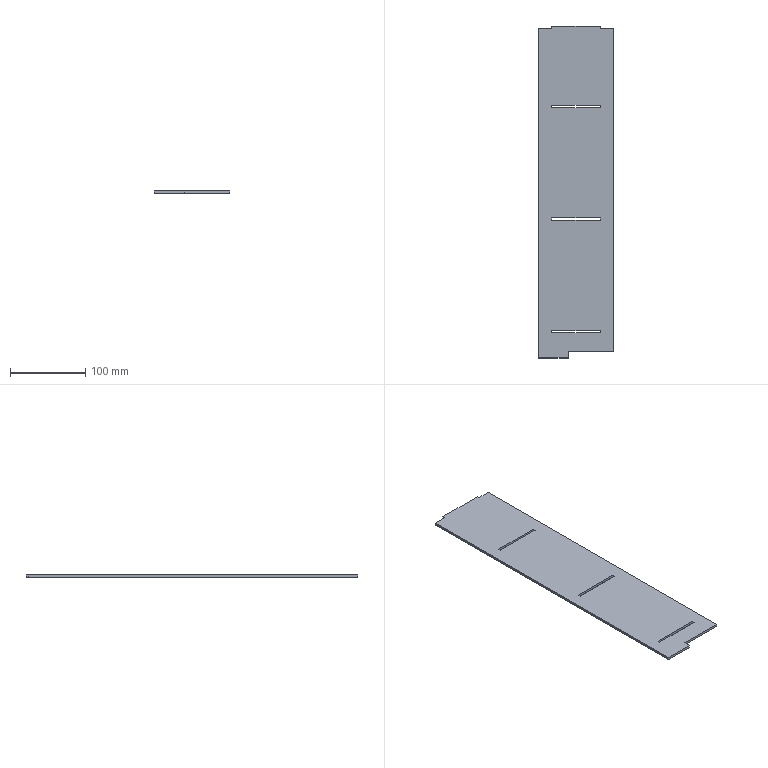Part | SolidWorks | features FlatPattern 1, SMBaseFlange 1, SheetMetal 1 | 1 solid | 24 faces | box 100 x 442 x 3.2 mm | volume 137506 mm3 | plane 24
STEP:
#1=CARTESIAN_POINT('',(72.5,-36.2,3.2));
#2=VERTEX_POINT('',#1);
#3=CARTESIAN_POINT('',(72.5,-33.,3.2));
#4=VERTEX_POINT('',#3);
#5=CARTESIAN_POINT('',(72.5,-33.,3.2));
#6=DIRECTION('',(0.,1.,0.));
#7=VECTOR('',#6,1000.);
#8=LINE('',#5,#7);
#9=EDGE_CURVE('',#2,#4,#8,.T.);
#10=ORIENTED_EDGE('',*,*,#9,.F.);
#11=CARTESIAN_POINT('',(7.5,-36.2,3.2));
#12=VERTEX_POINT('',#11);
#13=CARTESIAN_POINT('',(72.5,-36.2,3.2));
#14=DIRECTION('',(1.,0.,0.));
#15=VECTOR('',#14,1000.);
#16=LINE('',#13,#15);
#17=EDGE_CURVE('',#12,#2,#16,.T.);
#18=ORIENTED_EDGE('',*,*,#17,.F.);
#19=CARTESIAN_POINT('',(7.5,-33.,3.2));
#20=VERTEX_POINT('',#19);
#21=CARTESIAN_POINT('',(7.5,-33.,3.2));
#22=DIRECTION('',(0.,-1.,0.));
#23=VECTOR('',#22,1000.);
#24=LINE('',#21,#23);
#25=EDGE_CURVE('',#20,#12,#24,.T.);
#26=ORIENTED_EDGE('',*,*,#25,.F.);
#27=CARTESIAN_POINT('',(72.5,-33.,3.2));
#28=DIRECTION('',(-1.,0.,0.));
#29=VECTOR('',#28,1000.);
#30=LINE('',#27,#29);
#31=EDGE_CURVE('',#4,#20,#30,.T.);
#32=ORIENTED_EDGE('',*,*,#31,.F.);
#33=EDGE_LOOP('',(#10,#18,#26,#32));
#34=FACE_BOUND('',#33,.T.);
#35=CARTESIAN_POINT('',(7.5,222.5,3.2));
#36=VERTEX_POINT('',#35);
#37=CARTESIAN_POINT('',(7.5,219.5,3.2));
#38=VERTEX_POINT('',#37);
#39=CARTESIAN_POINT('',(7.5,219.5,3.2));
#40=DIRECTION('',(0.,-1.,0.));
#41=VECTOR('',#40,1000.);
#42=LINE('',#39,#41);
#43=EDGE_CURVE('',#36,#38,#42,.T.);
#44=ORIENTED_EDGE('',*,*,#43,.T.);
#45=CARTESIAN_POINT('',(-10.,219.5,3.2));
#46=VERTEX_POINT('',#45);
#47=CARTESIAN_POINT('',(-10.,219.5,3.2));
#48=DIRECTION('',(-1.,0.,0.));
#49=VECTOR('',#48,1000.);
#50=LINE('',#47,#49);
#51=EDGE_CURVE('',#38,#46,#50,.T.);
#52=ORIENTED_EDGE('',*,*,#51,.T.);
#53=CARTESIAN_POINT('',(-10.,-219.5,3.2));
#54=VERTEX_POINT('',#53);
#55=CARTESIAN_POINT('',(-10.,-219.5,3.2));
#56=DIRECTION('',(0.,-1.,0.));
#57=VECTOR('',#56,1000.);
#58=LINE('',#55,#57);
#59=EDGE_CURVE('',#46,#54,#58,.T.);
#60=ORIENTED_EDGE('',*,*,#59,.T.);
#61=CARTESIAN_POINT('',(29.7,-219.5,3.2));
#62=VERTEX_POINT('',#61);
#63=CARTESIAN_POINT('',(29.7,-219.5,3.2));
#64=DIRECTION('',(1.,0.,0.));
#65=VECTOR('',#64,1000.);
#66=LINE('',#63,#65);
#67=EDGE_CURVE('',#54,#62,#66,.T.);
#68=ORIENTED_EDGE('',*,*,#67,.T.);
#69=CARTESIAN_POINT('',(29.7,-211.2,3.2));
#70=VERTEX_POINT('',#69);
#71=CARTESIAN_POINT('',(29.7,-211.2,3.2));
#72=DIRECTION('',(0.,1.,0.));
#73=VECTOR('',#72,1000.);
#74=LINE('',#71,#73);
#75=EDGE_CURVE('',#62,#70,#74,.T.);
#76=ORIENTED_EDGE('',*,*,#75,.T.);
#77=CARTESIAN_POINT('',(90.,-211.2,3.2));
#78=VERTEX_POINT('',#77);
#79=CARTESIAN_POINT('',(90.,-211.2,3.2));
#80=DIRECTION('',(1.,0.,0.));
#81=VECTOR('',#80,1000.);
#82=LINE('',#79,#81);
#83=EDGE_CURVE('',#70,#78,#82,.T.);
#84=ORIENTED_EDGE('',*,*,#83,.T.);
#85=CARTESIAN_POINT('',(90.,219.5,3.2));
#86=VERTEX_POINT('',#85);
#87=CARTESIAN_POINT('',(90.,219.5,3.2));
#88=DIRECTION('',(0.,1.,0.));
#89=VECTOR('',#88,1000.);
#90=LINE('',#87,#89);
#91=EDGE_CURVE('',#78,#86,#90,.T.);
#92=ORIENTED_EDGE('',*,*,#91,.T.);
#93=CARTESIAN_POINT('',(72.5,219.5,3.2));
#94=VERTEX_POINT('',#93);
#95=CARTESIAN_POINT('',(72.5,219.5,3.2));
#96=DIRECTION('',(-1.,0.,0.));
#97=VECTOR('',#96,1000.);
#98=LINE('',#95,#97);
#99=EDGE_CURVE('',#86,#94,#98,.T.);
#100=ORIENTED_EDGE('',*,*,#99,.T.);
#101=CARTESIAN_POINT('',(72.5,222.5,3.2));
#102=VERTEX_POINT('',#101);
#103=CARTESIAN_POINT('',(72.5,222.5,3.2));
#104=DIRECTION('',(0.,1.,0.));
#105=VECTOR('',#104,1000.);
#106=LINE('',#103,#105);
#107=EDGE_CURVE('',#94,#102,#106,.T.);
#108=ORIENTED_EDGE('',*,*,#107,.T.);
#109=CARTESIAN_POINT('',(7.5,222.5,3.2));
#110=DIRECTION('',(-1.,0.,0.));
#111=VECTOR('',#110,1000.);
#112=LINE('',#109,#111);
#113=EDGE_CURVE('',#102,#36,#112,.T.);
#114=ORIENTED_EDGE('',*,*,#113,.T.);
#115=EDGE_LOOP('',(#44,#52,#60,#68,#76,#84,#92,#100,#108,#114));
#116=FACE_OUTER_BOUND('',#115,.T.);
#117=CARTESIAN_POINT('',(72.5,-186.2,3.2));
#118=VERTEX_POINT('',#117);
#119=CARTESIAN_POINT('',(72.5,-183.,3.2));
#120=VERTEX_POINT('',#119);
#121=CARTESIAN_POINT('',(72.5,-183.,3.2));
#122=DIRECTION('',(0.,1.,0.));
#123=VECTOR('',#122,1000.);
#124=LINE('',#121,#123);
#125=EDGE_CURVE('',#118,#120,#124,.T.);
#126=ORIENTED_EDGE('',*,*,#125,.F.);
#127=CARTESIAN_POINT('',(7.5,-186.2,3.2));
#128=VERTEX_POINT('',#127);
#129=CARTESIAN_POINT('',(72.5,-186.2,3.2));
#130=DIRECTION('',(1.,0.,0.));
#131=VECTOR('',#130,1000.);
#132=LINE('',#129,#131);
#133=EDGE_CURVE('',#128,#118,#132,.T.);
#134=ORIENTED_EDGE('',*,*,#133,.F.);
#135=CARTESIAN_POINT('',(7.5,-183.,3.2));
#136=VERTEX_POINT('',#135);
#137=CARTESIAN_POINT('',(7.5,-183.,3.2));
#138=DIRECTION('',(0.,-1.,0.));
#139=VECTOR('',#138,1000.);
#140=LINE('',#137,#139);
#141=EDGE_CURVE('',#136,#128,#140,.T.);
#142=ORIENTED_EDGE('',*,*,#141,.F.);
#143=CARTESIAN_POINT('',(72.5,-183.,3.2));
#144=DIRECTION('',(-1.,0.,0.));
#145=VECTOR('',#144,1000.);
#146=LINE('',#143,#145);
#147=EDGE_CURVE('',#120,#136,#146,.T.);
#148=ORIENTED_EDGE('',*,*,#147,.F.);
#149=EDGE_LOOP('',(#126,#134,#142,#148));
#150=FACE_BOUND('',#149,.T.);
#151=CARTESIAN_POINT('',(72.5,113.8,3.2));
#152=VERTEX_POINT('',#151);
#153=CARTESIAN_POINT('',(72.5,117.,3.2));
#154=VERTEX_POINT('',#153);
#155=CARTESIAN_POINT('',(72.5,117.,3.2));
#156=DIRECTION('',(0.,1.,0.));
#157=VECTOR('',#156,1000.);
#158=LINE('',#155,#157);
#159=EDGE_CURVE('',#152,#154,#158,.T.);
#160=ORIENTED_EDGE('',*,*,#159,.F.);
#161=CARTESIAN_POINT('',(7.5,113.8,3.2));
#162=VERTEX_POINT('',#161);
#163=CARTESIAN_POINT('',(72.5,113.8,3.2));
#164=DIRECTION('',(1.,0.,0.));
#165=VECTOR('',#164,1000.);
#166=LINE('',#163,#165);
#167=EDGE_CURVE('',#162,#152,#166,.T.);
#168=ORIENTED_EDGE('',*,*,#167,.F.);
#169=CARTESIAN_POINT('',(7.5,117.,3.2));
#170=VERTEX_POINT('',#169);
#171=CARTESIAN_POINT('',(7.5,117.,3.2));
#172=DIRECTION('',(0.,-1.,0.));
#173=VECTOR('',#172,1000.);
#174=LINE('',#171,#173);
#175=EDGE_CURVE('',#170,#162,#174,.T.);
#176=ORIENTED_EDGE('',*,*,#175,.F.);
#177=CARTESIAN_POINT('',(72.5,117.,3.2));
#178=DIRECTION('',(-1.,0.,0.));
#179=VECTOR('',#178,1000.);
#180=LINE('',#177,#179);
#181=EDGE_CURVE('',#154,#170,#180,.T.);
#182=ORIENTED_EDGE('',*,*,#181,.F.);
#183=EDGE_LOOP('',(#160,#168,#176,#182));
#184=FACE_BOUND('',#183,.T.);
#185=CARTESIAN_POINT('',(0.,0.,3.2));
#186=DIRECTION('',(0.,0.,-1.));
#187=DIRECTION('',(-1.,0.,0.));
#188=AXIS2_PLACEMENT_3D('',#185,#186,#187);
#189=PLANE('',#188);
#190=ADVANCED_FACE('',(#34,#116,#150,#184),#189,.F.);
#191=CARTESIAN_POINT('',(7.5,222.5,0.));
#192=VERTEX_POINT('',#191);
#193=CARTESIAN_POINT('',(7.5,219.5,0.));
#194=VERTEX_POINT('',#193);
#195=CARTESIAN_POINT('',(7.5,219.5,0.));
#196=DIRECTION('',(0.,-1.,0.));
#197=VECTOR('',#196,1000.);
#198=LINE('',#195,#197);
#199=EDGE_CURVE('',#192,#194,#198,.T.);
#200=ORIENTED_EDGE('',*,*,#199,.F.);
#201=CARTESIAN_POINT('',(72.5,222.5,0.));
#202=VERTEX_POINT('',#201);
#203=CARTESIAN_POINT('',(7.5,222.5,0.));
#204=DIRECTION('',(-1.,0.,0.));
#205=VECTOR('',#204,1000.);
#206=LINE('',#203,#205);
#207=EDGE_CURVE('',#202,#192,#206,.T.);
#208=ORIENTED_EDGE('',*,*,#207,.F.);
#209=CARTESIAN_POINT('',(72.5,219.5,0.));
#210=VERTEX_POINT('',#209);
#211=CARTESIAN_POINT('',(72.5,222.5,0.));
#212=DIRECTION('',(0.,1.,0.));
#213=VECTOR('',#212,1000.);
#214=LINE('',#211,#213);
#215=EDGE_CURVE('',#210,#202,#214,.T.);
#216=ORIENTED_EDGE('',*,*,#215,.F.);
#217=CARTESIAN_POINT('',(90.,219.5,0.));
#218=VERTEX_POINT('',#217);
#219=CARTESIAN_POINT('',(72.5,219.5,0.));
#220=DIRECTION('',(-1.,0.,0.));
#221=VECTOR('',#220,1000.);
#222=LINE('',#219,#221);
#223=EDGE_CURVE('',#218,#210,#222,.T.);
#224=ORIENTED_EDGE('',*,*,#223,.F.);
#225=CARTESIAN_POINT('',(90.,-211.2,0.));
#226=VERTEX_POINT('',#225);
#227=CARTESIAN_POINT('',(90.,219.5,0.));
#228=DIRECTION('',(0.,1.,0.));
#229=VECTOR('',#228,1000.);
#230=LINE('',#227,#229);
#231=EDGE_CURVE('',#226,#218,#230,.T.);
#232=ORIENTED_EDGE('',*,*,#231,.F.);
#233=CARTESIAN_POINT('',(29.7,-211.2,0.));
#234=VERTEX_POINT('',#233);
#235=CARTESIAN_POINT('',(90.,-211.2,0.));
#236=DIRECTION('',(1.,0.,0.));
#237=VECTOR('',#236,1000.);
#238=LINE('',#235,#237);
#239=EDGE_CURVE('',#234,#226,#238,.T.);
#240=ORIENTED_EDGE('',*,*,#239,.F.);
#241=CARTESIAN_POINT('',(29.7,-219.5,0.));
#242=VERTEX_POINT('',#241);
#243=CARTESIAN_POINT('',(29.7,-211.2,0.));
#244=DIRECTION('',(0.,1.,0.));
#245=VECTOR('',#244,1000.);
#246=LINE('',#243,#245);
#247=EDGE_CURVE('',#242,#234,#246,.T.);
#248=ORIENTED_EDGE('',*,*,#247,.F.);
#249=CARTESIAN_POINT('',(-10.,-219.5,0.));
#250=VERTEX_POINT('',#249);
#251=CARTESIAN_POINT('',(29.7,-219.5,0.));
#252=DIRECTION('',(1.,0.,0.));
#253=VECTOR('',#252,1000.);
#254=LINE('',#251,#253);
#255=EDGE_CURVE('',#250,#242,#254,.T.);
#256=ORIENTED_EDGE('',*,*,#255,.F.);
#257=CARTESIAN_POINT('',(-10.,219.5,0.));
#258=VERTEX_POINT('',#257);
#259=CARTESIAN_POINT('',(-10.,-219.5,0.));
#260=DIRECTION('',(0.,-1.,0.));
#261=VECTOR('',#260,1000.);
#262=LINE('',#259,#261);
#263=EDGE_CURVE('',#258,#250,#262,.T.);
#264=ORIENTED_EDGE('',*,*,#263,.F.);
#265=CARTESIAN_POINT('',(-10.,219.5,0.));
#266=DIRECTION('',(-1.,0.,0.));
#267=VECTOR('',#266,1000.);
#268=LINE('',#265,#267);
#269=EDGE_CURVE('',#194,#258,#268,.T.);
#270=ORIENTED_EDGE('',*,*,#269,.F.);
#271=EDGE_LOOP('',(#200,#208,#216,#224,#232,#240,#248,#256,#264,#270));
#272=FACE_OUTER_BOUND('',#271,.T.);
#273=CARTESIAN_POINT('',(7.5,-186.2,0.));
#274=VERTEX_POINT('',#273);
#275=CARTESIAN_POINT('',(72.5,-186.2,0.));
#276=VERTEX_POINT('',#275);
#277=CARTESIAN_POINT('',(72.5,-186.2,0.));
#278=DIRECTION('',(1.,0.,0.));
#279=VECTOR('',#278,1000.);
#280=LINE('',#277,#279);
#281=EDGE_CURVE('',#274,#276,#280,.T.);
#282=ORIENTED_EDGE('',*,*,#281,.T.);
#283=CARTESIAN_POINT('',(72.5,-183.,0.));
#284=VERTEX_POINT('',#283);
#285=CARTESIAN_POINT('',(72.5,-183.,0.));
#286=DIRECTION('',(0.,1.,0.));
#287=VECTOR('',#286,1000.);
#288=LINE('',#285,#287);
#289=EDGE_CURVE('',#276,#284,#288,.T.);
#290=ORIENTED_EDGE('',*,*,#289,.T.);
#291=CARTESIAN_POINT('',(7.5,-183.,0.));
#292=VERTEX_POINT('',#291);
#293=CARTESIAN_POINT('',(72.5,-183.,0.));
#294=DIRECTION('',(-1.,0.,0.));
#295=VECTOR('',#294,1000.);
#296=LINE('',#293,#295);
#297=EDGE_CURVE('',#284,#292,#296,.T.);
#298=ORIENTED_EDGE('',*,*,#297,.T.);
#299=CARTESIAN_POINT('',(7.5,-183.,0.));
#300=DIRECTION('',(0.,-1.,0.));
#301=VECTOR('',#300,1000.);
#302=LINE('',#299,#301);
#303=EDGE_CURVE('',#292,#274,#302,.T.);
#304=ORIENTED_EDGE('',*,*,#303,.T.);
#305=EDGE_LOOP('',(#282,#290,#298,#304));
#306=FACE_BOUND('',#305,.T.);
#307=CARTESIAN_POINT('',(7.5,-36.2,0.));
#308=VERTEX_POINT('',#307);
#309=CARTESIAN_POINT('',(72.5,-36.2,0.));
#310=VERTEX_POINT('',#309);
#311=CARTESIAN_POINT('',(72.5,-36.2,0.));
#312=DIRECTION('',(1.,0.,0.));
#313=VECTOR('',#312,1000.);
#314=LINE('',#311,#313);
#315=EDGE_CURVE('',#308,#310,#314,.T.);
#316=ORIENTED_EDGE('',*,*,#315,.T.);
#317=CARTESIAN_POINT('',(72.5,-33.,0.));
#318=VERTEX_POINT('',#317);
#319=CARTESIAN_POINT('',(72.5,-33.,0.));
#320=DIRECTION('',(0.,1.,0.));
#321=VECTOR('',#320,1000.);
#322=LINE('',#319,#321);
#323=EDGE_CURVE('',#310,#318,#322,.T.);
#324=ORIENTED_EDGE('',*,*,#323,.T.);
#325=CARTESIAN_POINT('',(7.5,-33.,0.));
#326=VERTEX_POINT('',#325);
#327=CARTESIAN_POINT('',(72.5,-33.,0.));
#328=DIRECTION('',(-1.,0.,0.));
#329=VECTOR('',#328,1000.);
#330=LINE('',#327,#329);
#331=EDGE_CURVE('',#318,#326,#330,.T.);
#332=ORIENTED_EDGE('',*,*,#331,.T.);
#333=CARTESIAN_POINT('',(7.5,-33.,0.));
#334=DIRECTION('',(0.,-1.,0.));
#335=VECTOR('',#334,1000.);
#336=LINE('',#333,#335);
#337=EDGE_CURVE('',#326,#308,#336,.T.);
#338=ORIENTED_EDGE('',*,*,#337,.T.);
#339=EDGE_LOOP('',(#316,#324,#332,#338));
#340=FACE_BOUND('',#339,.T.);
#341=CARTESIAN_POINT('',(7.5,113.8,0.));
#342=VERTEX_POINT('',#341);
#343=CARTESIAN_POINT('',(72.5,113.8,0.));
#344=VERTEX_POINT('',#343);
#345=CARTESIAN_POINT('',(72.5,113.8,0.));
#346=DIRECTION('',(1.,0.,0.));
#347=VECTOR('',#346,1000.);
#348=LINE('',#345,#347);
#349=EDGE_CURVE('',#342,#344,#348,.T.);
#350=ORIENTED_EDGE('',*,*,#349,.T.);
#351=CARTESIAN_POINT('',(72.5,117.,0.));
#352=VERTEX_POINT('',#351);
#353=CARTESIAN_POINT('',(72.5,117.,0.));
#354=DIRECTION('',(0.,1.,0.));
#355=VECTOR('',#354,1000.);
#356=LINE('',#353,#355);
#357=EDGE_CURVE('',#344,#352,#356,.T.);
#358=ORIENTED_EDGE('',*,*,#357,.T.);
#359=CARTESIAN_POINT('',(7.5,117.,0.));
#360=VERTEX_POINT('',#359);
#361=CARTESIAN_POINT('',(72.5,117.,0.));
#362=DIRECTION('',(-1.,0.,0.));
#363=VECTOR('',#362,1000.);
#364=LINE('',#361,#363);
#365=EDGE_CURVE('',#352,#360,#364,.T.);
#366=ORIENTED_EDGE('',*,*,#365,.T.);
#367=CARTESIAN_POINT('',(7.5,117.,0.));
#368=DIRECTION('',(0.,-1.,0.));
#369=VECTOR('',#368,1000.);
#370=LINE('',#367,#369);
#371=EDGE_CURVE('',#360,#342,#370,.T.);
#372=ORIENTED_EDGE('',*,*,#371,.T.);
#373=EDGE_LOOP('',(#350,#358,#366,#372));
#374=FACE_BOUND('',#373,.T.);
#375=CARTESIAN_POINT('',(0.,0.,0.));
#376=DIRECTION('',(0.,0.,-1.));
#377=DIRECTION('',(-1.,0.,0.));
#378=AXIS2_PLACEMENT_3D('',#375,#376,#377);
#379=PLANE('',#378);
#380=ADVANCED_FACE('',(#272,#306,#340,#374),#379,.T.);
#381=ORIENTED_EDGE('',*,*,#199,.T.);
#382=CARTESIAN_POINT('',(7.5,219.5,3.2));
#383=DIRECTION('',(0.,0.,-1.));
#384=VECTOR('',#383,1000.);
#385=LINE('',#382,#384);
#386=EDGE_CURVE('',#38,#194,#385,.T.);
#387=ORIENTED_EDGE('',*,*,#386,.F.);
#388=ORIENTED_EDGE('',*,*,#43,.F.);
#389=CARTESIAN_POINT('',(7.5,222.5,3.2));
#390=DIRECTION('',(0.,0.,-1.));
#391=VECTOR('',#390,1000.);
#392=LINE('',#389,#391);
#393=EDGE_CURVE('',#36,#192,#392,.T.);
#394=ORIENTED_EDGE('',*,*,#393,.T.);
#395=EDGE_LOOP('',(#381,#387,#388,#394));
#396=FACE_OUTER_BOUND('',#395,.T.);
#397=CARTESIAN_POINT('',(7.5,219.5,3.2));
#398=DIRECTION('',(1.,0.,0.));
#399=DIRECTION('',(0.,1.,0.));
#400=AXIS2_PLACEMENT_3D('',#397,#398,#399);
#401=PLANE('',#400);
#402=ADVANCED_FACE('',(#396),#401,.F.);
#403=ORIENTED_EDGE('',*,*,#269,.T.);
#404=CARTESIAN_POINT('',(-10.,219.5,3.2));
#405=DIRECTION('',(0.,0.,-1.));
#406=VECTOR('',#405,1000.);
#407=LINE('',#404,#406);
#408=EDGE_CURVE('',#46,#258,#407,.T.);
#409=ORIENTED_EDGE('',*,*,#408,.F.);
#410=ORIENTED_EDGE('',*,*,#51,.F.);
#411=ORIENTED_EDGE('',*,*,#386,.T.);
#412=EDGE_LOOP('',(#403,#409,#410,#411));
#413=FACE_OUTER_BOUND('',#412,.T.);
#414=CARTESIAN_POINT('',(-10.,219.5,3.2));
#415=DIRECTION('',(0.,-1.,0.));
#416=DIRECTION('',(0.,0.,-1.));
#417=AXIS2_PLACEMENT_3D('',#414,#415,#416);
#418=PLANE('',#417);
#419=ADVANCED_FACE('',(#413),#418,.F.);
#420=ORIENTED_EDGE('',*,*,#263,.T.);
#421=CARTESIAN_POINT('',(-10.,-219.5,3.2));
#422=DIRECTION('',(0.,0.,-1.));
#423=VECTOR('',#422,1000.);
#424=LINE('',#421,#423);
#425=EDGE_CURVE('',#54,#250,#424,.T.);
#426=ORIENTED_EDGE('',*,*,#425,.F.);
#427=ORIENTED_EDGE('',*,*,#59,.F.);
#428=ORIENTED_EDGE('',*,*,#408,.T.);
#429=EDGE_LOOP('',(#420,#426,#427,#428));
#430=FACE_OUTER_BOUND('',#429,.T.);
#431=CARTESIAN_POINT('',(-10.,-219.5,3.2));
#432=DIRECTION('',(1.,0.,0.));
#433=DIRECTION('',(0.,0.,-1.));
#434=AXIS2_PLACEMENT_3D('',#431,#432,#433);
#435=PLANE('',#434);
#436=ADVANCED_FACE('',(#430),#435,.F.);
#437=ORIENTED_EDGE('',*,*,#255,.T.);
#438=CARTESIAN_POINT('',(29.7,-219.5,3.2));
#439=DIRECTION('',(0.,0.,-1.));
#440=VECTOR('',#439,1000.);
#441=LINE('',#438,#440);
#442=EDGE_CURVE('',#62,#242,#441,.T.);
#443=ORIENTED_EDGE('',*,*,#442,.F.);
#444=ORIENTED_EDGE('',*,*,#67,.F.);
#445=ORIENTED_EDGE('',*,*,#425,.T.);
#446=EDGE_LOOP('',(#437,#443,#444,#445));
#447=FACE_OUTER_BOUND('',#446,.T.);
#448=CARTESIAN_POINT('',(29.7,-219.5,3.2));
#449=DIRECTION('',(0.,1.,0.));
#450=DIRECTION('',(0.,0.,1.));
#451=AXIS2_PLACEMENT_3D('',#448,#449,#450);
#452=PLANE('',#451);
#453=ADVANCED_FACE('',(#447),#452,.F.);
#454=ORIENTED_EDGE('',*,*,#247,.T.);
#455=CARTESIAN_POINT('',(29.7,-211.2,3.2));
#456=DIRECTION('',(0.,0.,-1.));
#457=VECTOR('',#456,1000.);
#458=LINE('',#455,#457);
#459=EDGE_CURVE('',#70,#234,#458,.T.);
#460=ORIENTED_EDGE('',*,*,#459,.F.);
#461=ORIENTED_EDGE('',*,*,#75,.F.);
#462=ORIENTED_EDGE('',*,*,#442,.T.);
#463=EDGE_LOOP('',(#454,#460,#461,#462));
#464=FACE_OUTER_BOUND('',#463,.T.);
#465=CARTESIAN_POINT('',(29.7,-211.2,3.2));
#466=DIRECTION('',(-1.,0.,0.));
#467=DIRECTION('',(0.,0.,1.));
#468=AXIS2_PLACEMENT_3D('',#465,#466,#467);
#469=PLANE('',#468);
#470=ADVANCED_FACE('',(#464),#469,.F.);
#471=ORIENTED_EDGE('',*,*,#239,.T.);
#472=CARTESIAN_POINT('',(90.,-211.2,3.2));
#473=DIRECTION('',(0.,0.,-1.));
#474=VECTOR('',#473,1000.);
#475=LINE('',#472,#474);
#476=EDGE_CURVE('',#78,#226,#475,.T.);
#477=ORIENTED_EDGE('',*,*,#476,.F.);
#478=ORIENTED_EDGE('',*,*,#83,.F.);
#479=ORIENTED_EDGE('',*,*,#459,.T.);
#480=EDGE_LOOP('',(#471,#477,#478,#479));
#481=FACE_OUTER_BOUND('',#480,.T.);
#482=CARTESIAN_POINT('',(90.,-211.2,3.2));
#483=DIRECTION('',(0.,1.,0.));
#484=DIRECTION('',(0.,0.,1.));
#485=AXIS2_PLACEMENT_3D('',#482,#483,#484);
#486=PLANE('',#485);
#487=ADVANCED_FACE('',(#481),#486,.F.);
#488=ORIENTED_EDGE('',*,*,#231,.T.);
#489=CARTESIAN_POINT('',(90.,219.5,3.2));
#490=DIRECTION('',(0.,0.,-1.));
#491=VECTOR('',#490,1000.);
#492=LINE('',#489,#491);
#493=EDGE_CURVE('',#86,#218,#492,.T.);
#494=ORIENTED_EDGE('',*,*,#493,.F.);
#495=ORIENTED_EDGE('',*,*,#91,.F.);
#496=ORIENTED_EDGE('',*,*,#476,.T.);
#497=EDGE_LOOP('',(#488,#494,#495,#496));
#498=FACE_OUTER_BOUND('',#497,.T.);
#499=CARTESIAN_POINT('',(90.,219.5,3.2));
#500=DIRECTION('',(-1.,0.,0.));
#501=DIRECTION('',(0.,-1.,0.));
#502=AXIS2_PLACEMENT_3D('',#499,#500,#501);
#503=PLANE('',#502);
#504=ADVANCED_FACE('',(#498),#503,.F.);
#505=ORIENTED_EDGE('',*,*,#223,.T.);
#506=CARTESIAN_POINT('',(72.5,219.5,3.2));
#507=DIRECTION('',(0.,0.,-1.));
#508=VECTOR('',#507,1000.);
#509=LINE('',#506,#508);
#510=EDGE_CURVE('',#94,#210,#509,.T.);
#511=ORIENTED_EDGE('',*,*,#510,.F.);
#512=ORIENTED_EDGE('',*,*,#99,.F.);
#513=ORIENTED_EDGE('',*,*,#493,.T.);
#514=EDGE_LOOP('',(#505,#511,#512,#513));
#515=FACE_OUTER_BOUND('',#514,.T.);
#516=CARTESIAN_POINT('',(72.5,219.5,3.2));
#517=DIRECTION('',(0.,-1.,0.));
#518=DIRECTION('',(0.,0.,-1.));
#519=AXIS2_PLACEMENT_3D('',#516,#517,#518);
#520=PLANE('',#519);
#521=ADVANCED_FACE('',(#515),#520,.F.);
#522=ORIENTED_EDGE('',*,*,#215,.T.);
#523=CARTESIAN_POINT('',(72.5,222.5,3.2));
#524=DIRECTION('',(0.,0.,-1.));
#525=VECTOR('',#524,1000.);
#526=LINE('',#523,#525);
#527=EDGE_CURVE('',#102,#202,#526,.T.);
#528=ORIENTED_EDGE('',*,*,#527,.F.);
#529=ORIENTED_EDGE('',*,*,#107,.F.);
#530=ORIENTED_EDGE('',*,*,#510,.T.);
#531=EDGE_LOOP('',(#522,#528,#529,#530));
#532=FACE_OUTER_BOUND('',#531,.T.);
#533=CARTESIAN_POINT('',(72.5,222.5,3.2));
#534=DIRECTION('',(-1.,0.,0.));
#535=DIRECTION('',(0.,0.,1.));
#536=AXIS2_PLACEMENT_3D('',#533,#534,#535);
#537=PLANE('',#536);
#538=ADVANCED_FACE('',(#532),#537,.F.);
#539=ORIENTED_EDGE('',*,*,#207,.T.);
#540=ORIENTED_EDGE('',*,*,#393,.F.);
#541=ORIENTED_EDGE('',*,*,#113,.F.);
#542=ORIENTED_EDGE('',*,*,#527,.T.);
#543=EDGE_LOOP('',(#539,#540,#541,#542));
#544=FACE_OUTER_BOUND('',#543,.T.);
#545=CARTESIAN_POINT('',(7.5,222.5,3.2));
#546=DIRECTION('',(0.,-1.,0.));
#547=DIRECTION('',(0.,0.,-1.));
#548=AXIS2_PLACEMENT_3D('',#545,#546,#547);
#549=PLANE('',#548);
#550=ADVANCED_FACE('',(#544),#549,.F.);
#551=ORIENTED_EDGE('',*,*,#289,.F.);
#552=CARTESIAN_POINT('',(72.5,-186.2,3.2));
#553=DIRECTION('',(0.,0.,-1.));
#554=VECTOR('',#553,1000.);
#555=LINE('',#552,#554);
#556=EDGE_CURVE('',#118,#276,#555,.T.);
#557=ORIENTED_EDGE('',*,*,#556,.F.);
#558=ORIENTED_EDGE('',*,*,#125,.T.);
#559=CARTESIAN_POINT('',(72.5,-183.,3.2));
#560=DIRECTION('',(0.,0.,-1.));
#561=VECTOR('',#560,1000.);
#562=LINE('',#559,#561);
#563=EDGE_CURVE('',#120,#284,#562,.T.);
#564=ORIENTED_EDGE('',*,*,#563,.T.);
#565=EDGE_LOOP('',(#551,#557,#558,#564));
#566=FACE_OUTER_BOUND('',#565,.T.);
#567=CARTESIAN_POINT('',(72.5,-183.,3.2));
#568=DIRECTION('',(-1.,0.,0.));
#569=DIRECTION('',(0.,0.,1.));
#570=AXIS2_PLACEMENT_3D('',#567,#568,#569);
#571=PLANE('',#570);
#572=ADVANCED_FACE('',(#566),#571,.T.);
#573=ORIENTED_EDGE('',*,*,#297,.F.);
#574=ORIENTED_EDGE('',*,*,#563,.F.);
#575=ORIENTED_EDGE('',*,*,#147,.T.);
#576=CARTESIAN_POINT('',(7.5,-183.,3.2));
#577=DIRECTION('',(0.,0.,-1.));
#578=VECTOR('',#577,1000.);
#579=LINE('',#576,#578);
#580=EDGE_CURVE('',#136,#292,#579,.T.);
#581=ORIENTED_EDGE('',*,*,#580,.T.);
#582=EDGE_LOOP('',(#573,#574,#575,#581));
#583=FACE_OUTER_BOUND('',#582,.T.);
#584=CARTESIAN_POINT('',(72.5,-183.,3.2));
#585=DIRECTION('',(0.,-1.,0.));
#586=DIRECTION('',(0.,0.,-1.));
#587=AXIS2_PLACEMENT_3D('',#584,#585,#586);
#588=PLANE('',#587);
#589=ADVANCED_FACE('',(#583),#588,.T.);
#590=ORIENTED_EDGE('',*,*,#303,.F.);
#591=ORIENTED_EDGE('',*,*,#580,.F.);
#592=ORIENTED_EDGE('',*,*,#141,.T.);
#593=CARTESIAN_POINT('',(7.5,-186.2,3.2));
#594=DIRECTION('',(0.,0.,-1.));
#595=VECTOR('',#594,1000.);
#596=LINE('',#593,#595);
#597=EDGE_CURVE('',#128,#274,#596,.T.);
#598=ORIENTED_EDGE('',*,*,#597,.T.);
#599=EDGE_LOOP('',(#590,#591,#592,#598));
#600=FACE_OUTER_BOUND('',#599,.T.);
#601=CARTESIAN_POINT('',(7.5,-183.,3.2));
#602=DIRECTION('',(1.,0.,0.));
#603=DIRECTION('',(0.,0.,-1.));
#604=AXIS2_PLACEMENT_3D('',#601,#602,#603);
#605=PLANE('',#604);
#606=ADVANCED_FACE('',(#600),#605,.T.);
#607=ORIENTED_EDGE('',*,*,#281,.F.);
#608=ORIENTED_EDGE('',*,*,#597,.F.);
#609=ORIENTED_EDGE('',*,*,#133,.T.);
#610=ORIENTED_EDGE('',*,*,#556,.T.);
#611=EDGE_LOOP('',(#607,#608,#609,#610));
#612=FACE_OUTER_BOUND('',#611,.T.);
#613=CARTESIAN_POINT('',(72.5,-186.2,3.2));
#614=DIRECTION('',(0.,1.,0.));
#615=DIRECTION('',(0.,0.,1.));
#616=AXIS2_PLACEMENT_3D('',#613,#614,#615);
#617=PLANE('',#616);
#618=ADVANCED_FACE('',(#612),#617,.T.);
#619=ORIENTED_EDGE('',*,*,#323,.F.);
#620=CARTESIAN_POINT('',(72.5,-36.2,3.2));
#621=DIRECTION('',(0.,0.,-1.));
#622=VECTOR('',#621,1000.);
#623=LINE('',#620,#622);
#624=EDGE_CURVE('',#2,#310,#623,.T.);
#625=ORIENTED_EDGE('',*,*,#624,.F.);
#626=ORIENTED_EDGE('',*,*,#9,.T.);
#627=CARTESIAN_POINT('',(72.5,-33.,3.2));
#628=DIRECTION('',(0.,0.,-1.));
#629=VECTOR('',#628,1000.);
#630=LINE('',#627,#629);
#631=EDGE_CURVE('',#4,#318,#630,.T.);
#632=ORIENTED_EDGE('',*,*,#631,.T.);
#633=EDGE_LOOP('',(#619,#625,#626,#632));
#634=FACE_OUTER_BOUND('',#633,.T.);
#635=CARTESIAN_POINT('',(72.5,-33.,3.2));
#636=DIRECTION('',(-1.,0.,0.));
#637=DIRECTION('',(0.,0.,1.));
#638=AXIS2_PLACEMENT_3D('',#635,#636,#637);
#639=PLANE('',#638);
#640=ADVANCED_FACE('',(#634),#639,.T.);
#641=ORIENTED_EDGE('',*,*,#331,.F.);
#642=ORIENTED_EDGE('',*,*,#631,.F.);
#643=ORIENTED_EDGE('',*,*,#31,.T.);
#644=CARTESIAN_POINT('',(7.5,-33.,3.2));
#645=DIRECTION('',(0.,0.,-1.));
#646=VECTOR('',#645,1000.);
#647=LINE('',#644,#646);
#648=EDGE_CURVE('',#20,#326,#647,.T.);
#649=ORIENTED_EDGE('',*,*,#648,.T.);
#650=EDGE_LOOP('',(#641,#642,#643,#649));
#651=FACE_OUTER_BOUND('',#650,.T.);
#652=CARTESIAN_POINT('',(72.5,-33.,3.2));
#653=DIRECTION('',(0.,-1.,0.));
#654=DIRECTION('',(0.,0.,-1.));
#655=AXIS2_PLACEMENT_3D('',#652,#653,#654);
#656=PLANE('',#655);
#657=ADVANCED_FACE('',(#651),#656,.T.);
#658=ORIENTED_EDGE('',*,*,#337,.F.);
#659=ORIENTED_EDGE('',*,*,#648,.F.);
#660=ORIENTED_EDGE('',*,*,#25,.T.);
#661=CARTESIAN_POINT('',(7.5,-36.2,3.2));
#662=DIRECTION('',(0.,0.,-1.));
#663=VECTOR('',#662,1000.);
#664=LINE('',#661,#663);
#665=EDGE_CURVE('',#12,#308,#664,.T.);
#666=ORIENTED_EDGE('',*,*,#665,.T.);
#667=EDGE_LOOP('',(#658,#659,#660,#666));
#668=FACE_OUTER_BOUND('',#667,.T.);
#669=CARTESIAN_POINT('',(7.5,-33.,3.2));
#670=DIRECTION('',(1.,0.,0.));
#671=DIRECTION('',(0.,0.,-1.));
#672=AXIS2_PLACEMENT_3D('',#669,#670,#671);
#673=PLANE('',#672);
#674=ADVANCED_FACE('',(#668),#673,.T.);
#675=ORIENTED_EDGE('',*,*,#315,.F.);
#676=ORIENTED_EDGE('',*,*,#665,.F.);
#677=ORIENTED_EDGE('',*,*,#17,.T.);
#678=ORIENTED_EDGE('',*,*,#624,.T.);
#679=EDGE_LOOP('',(#675,#676,#677,#678));
#680=FACE_OUTER_BOUND('',#679,.T.);
#681=CARTESIAN_POINT('',(72.5,-36.2,3.2));
#682=DIRECTION('',(0.,1.,0.));
#683=DIRECTION('',(0.,0.,1.));
#684=AXIS2_PLACEMENT_3D('',#681,#682,#683);
#685=PLANE('',#684);
#686=ADVANCED_FACE('',(#680),#685,.T.);
#687=ORIENTED_EDGE('',*,*,#357,.F.);
#688=CARTESIAN_POINT('',(72.5,113.8,3.2));
#689=DIRECTION('',(0.,0.,-1.));
#690=VECTOR('',#689,1000.);
#691=LINE('',#688,#690);
#692=EDGE_CURVE('',#152,#344,#691,.T.);
#693=ORIENTED_EDGE('',*,*,#692,.F.);
#694=ORIENTED_EDGE('',*,*,#159,.T.);
#695=CARTESIAN_POINT('',(72.5,117.,3.2));
#696=DIRECTION('',(0.,0.,-1.));
#697=VECTOR('',#696,1000.);
#698=LINE('',#695,#697);
#699=EDGE_CURVE('',#154,#352,#698,.T.);
#700=ORIENTED_EDGE('',*,*,#699,.T.);
#701=EDGE_LOOP('',(#687,#693,#694,#700));
#702=FACE_OUTER_BOUND('',#701,.T.);
#703=CARTESIAN_POINT('',(72.5,117.,3.2));
#704=DIRECTION('',(-1.,0.,0.));
#705=DIRECTION('',(0.,0.,1.));
#706=AXIS2_PLACEMENT_3D('',#703,#704,#705);
#707=PLANE('',#706);
#708=ADVANCED_FACE('',(#702),#707,.T.);
#709=ORIENTED_EDGE('',*,*,#365,.F.);
#710=ORIENTED_EDGE('',*,*,#699,.F.);
#711=ORIENTED_EDGE('',*,*,#181,.T.);
#712=CARTESIAN_POINT('',(7.5,117.,3.2));
#713=DIRECTION('',(0.,0.,-1.));
#714=VECTOR('',#713,1000.);
#715=LINE('',#712,#714);
#716=EDGE_CURVE('',#170,#360,#715,.T.);
#717=ORIENTED_EDGE('',*,*,#716,.T.);
#718=EDGE_LOOP('',(#709,#710,#711,#717));
#719=FACE_OUTER_BOUND('',#718,.T.);
#720=CARTESIAN_POINT('',(72.5,117.,3.2));
#721=DIRECTION('',(0.,-1.,0.));
#722=DIRECTION('',(0.,0.,-1.));
#723=AXIS2_PLACEMENT_3D('',#720,#721,#722);
#724=PLANE('',#723);
#725=ADVANCED_FACE('',(#719),#724,.T.);
#726=ORIENTED_EDGE('',*,*,#371,.F.);
#727=ORIENTED_EDGE('',*,*,#716,.F.);
#728=ORIENTED_EDGE('',*,*,#175,.T.);
#729=CARTESIAN_POINT('',(7.5,113.8,3.2));
#730=DIRECTION('',(0.,0.,-1.));
#731=VECTOR('',#730,1000.);
#732=LINE('',#729,#731);
#733=EDGE_CURVE('',#162,#342,#732,.T.);
#734=ORIENTED_EDGE('',*,*,#733,.T.);
#735=EDGE_LOOP('',(#726,#727,#728,#734));
#736=FACE_OUTER_BOUND('',#735,.T.);
#737=CARTESIAN_POINT('',(7.5,117.,3.2));
#738=DIRECTION('',(1.,0.,0.));
#739=DIRECTION('',(0.,0.,-1.));
#740=AXIS2_PLACEMENT_3D('',#737,#738,#739);
#741=PLANE('',#740);
#742=ADVANCED_FACE('',(#736),#741,.T.);
#743=ORIENTED_EDGE('',*,*,#349,.F.);
#744=ORIENTED_EDGE('',*,*,#733,.F.);
#745=ORIENTED_EDGE('',*,*,#167,.T.);
#746=ORIENTED_EDGE('',*,*,#692,.T.);
#747=EDGE_LOOP('',(#743,#744,#745,#746));
#748=FACE_OUTER_BOUND('',#747,.T.);
#749=CARTESIAN_POINT('',(72.5,113.8,3.2));
#750=DIRECTION('',(0.,1.,0.));
#751=DIRECTION('',(0.,0.,1.));
#752=AXIS2_PLACEMENT_3D('',#749,#750,#751);
#753=PLANE('',#752);
#754=ADVANCED_FACE('',(#748),#753,.T.);
#755=CLOSED_SHELL('',(#190,#380,#402,#419,#436,#453,#470,#487,#504,#521,#538,#550,#572,#589,#606,#618,#640,#657,#674,#686,#708,#725,#742,#754));
#756=MANIFOLD_SOLID_BREP('',#755);
#757=CARTESIAN_POINT('',(0.,0.,0.));
#758=DIRECTION('',(0.,0.,1.));
#759=DIRECTION('',(1.,0.,0.));
#760=AXIS2_PLACEMENT_3D('',#757,#758,#759);
#761=(LENGTH_UNIT()NAMED_UNIT(*)SI_UNIT(.MILLI.,.METRE.));
#762=UNCERTAINTY_MEASURE_WITH_UNIT(LENGTH_MEASURE(0.00001),#761,'','');
#763=(NAMED_UNIT(*)PLANE_ANGLE_UNIT()SI_UNIT($,.RADIAN.));
#764=(NAMED_UNIT(*)SI_UNIT($,.STERADIAN.)SOLID_ANGLE_UNIT());
#765=(GEOMETRIC_REPRESENTATION_CONTEXT(3)GLOBAL_UNCERTAINTY_ASSIGNED_CONTEXT((#762))GLOBAL_UNIT_ASSIGNED_CONTEXT((#761,#763,#764))REPRESENTATION_CONTEXT('',''));
#766=ADVANCED_BREP_SHAPE_REPRESENTATION('',(#756,#760),#765);